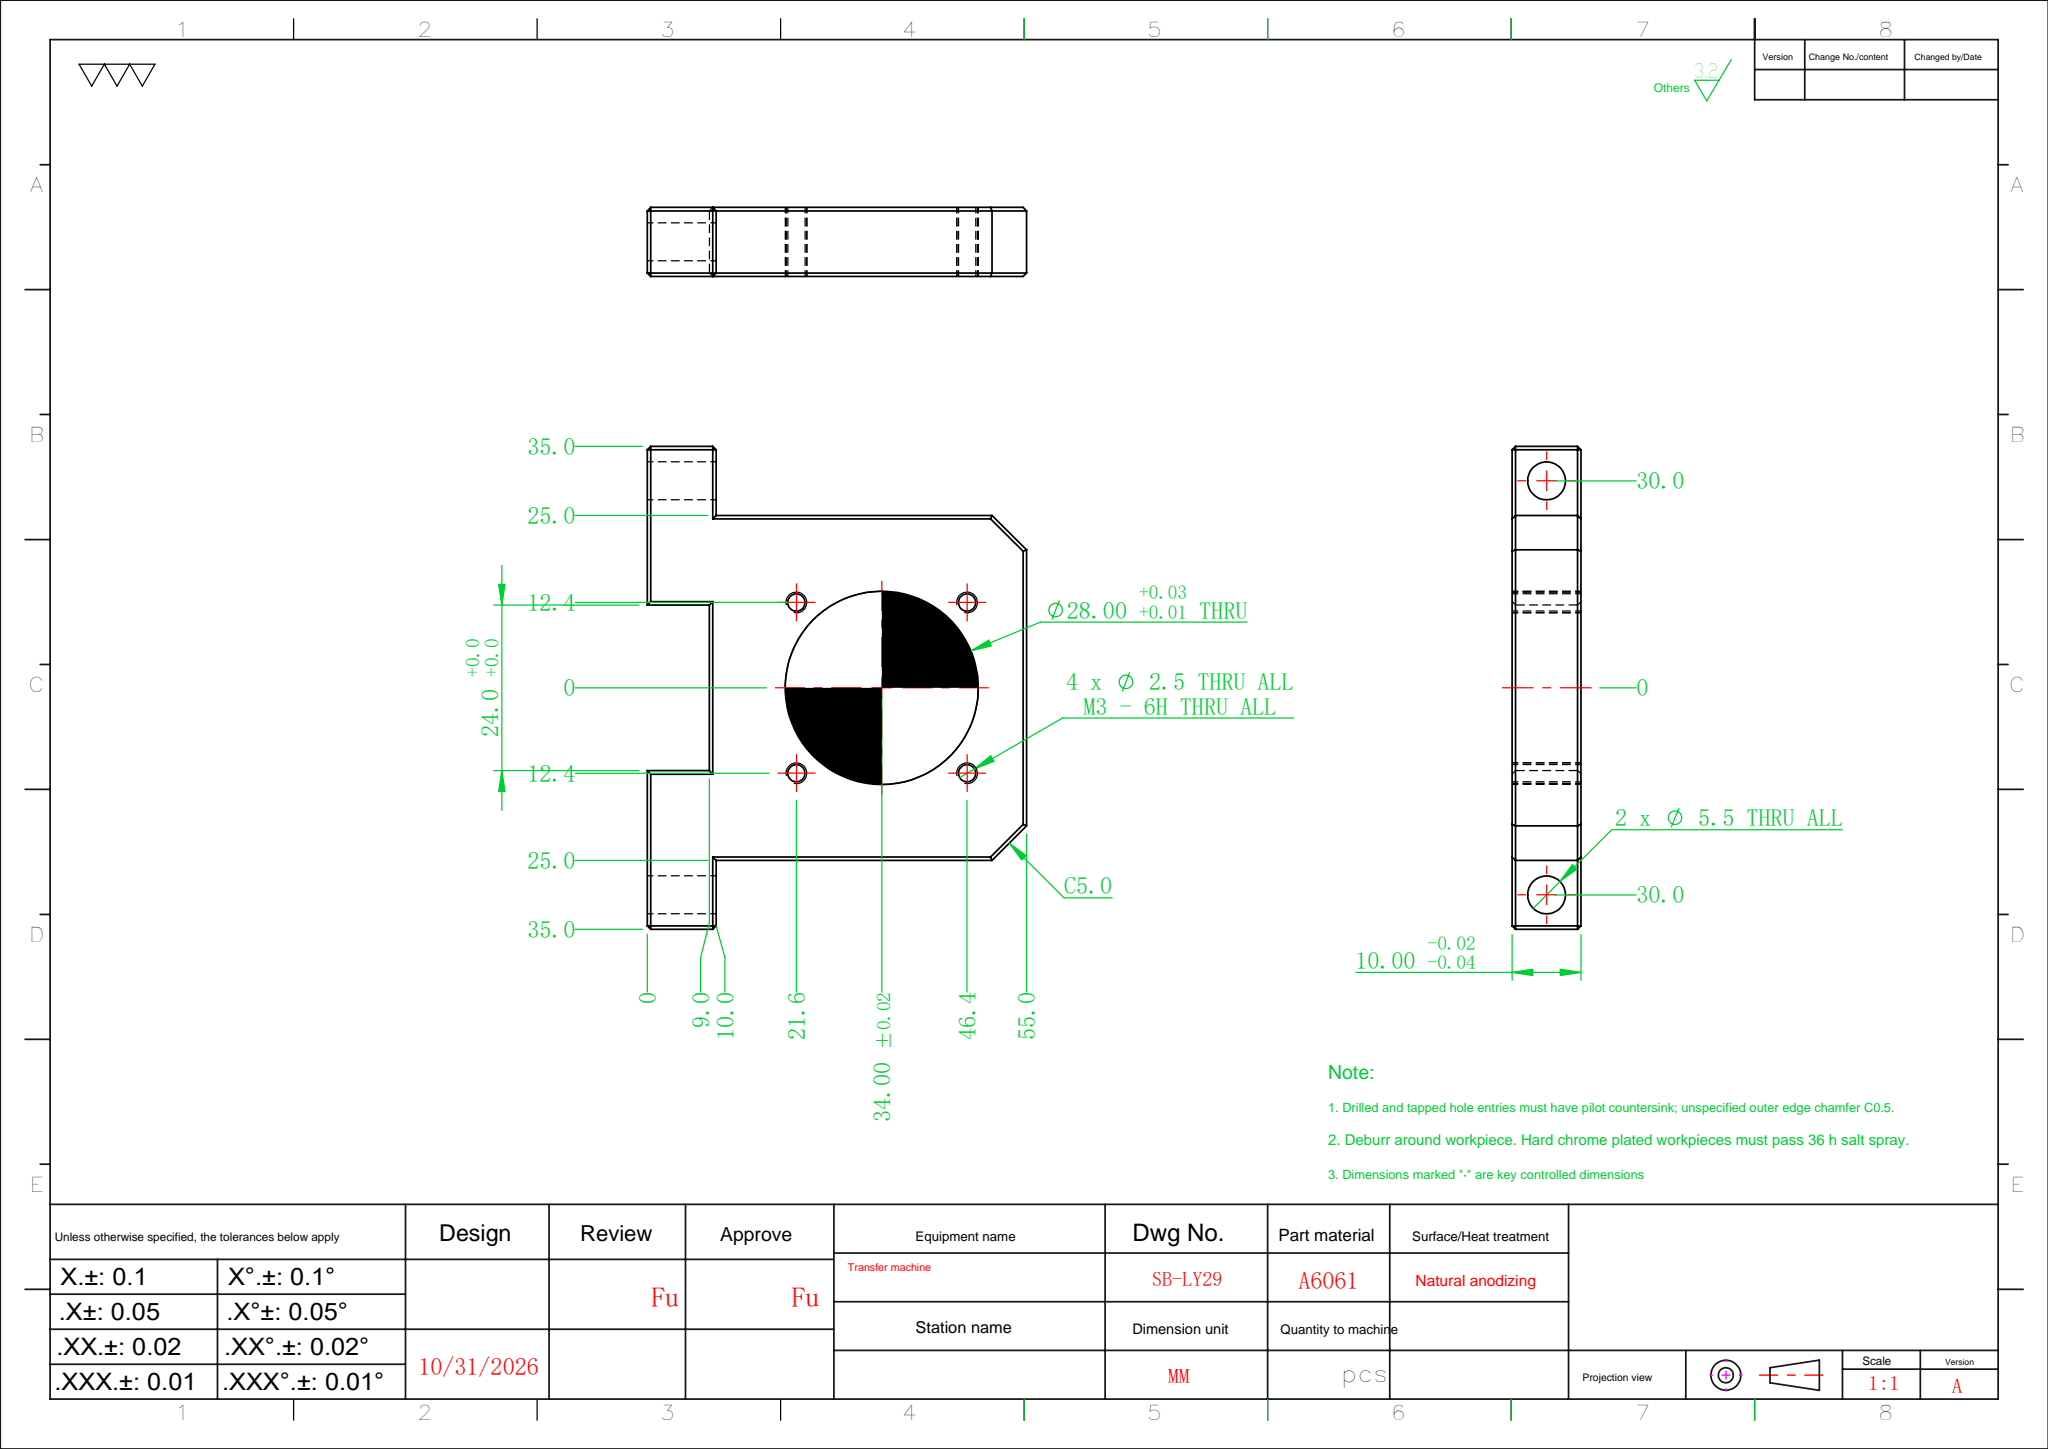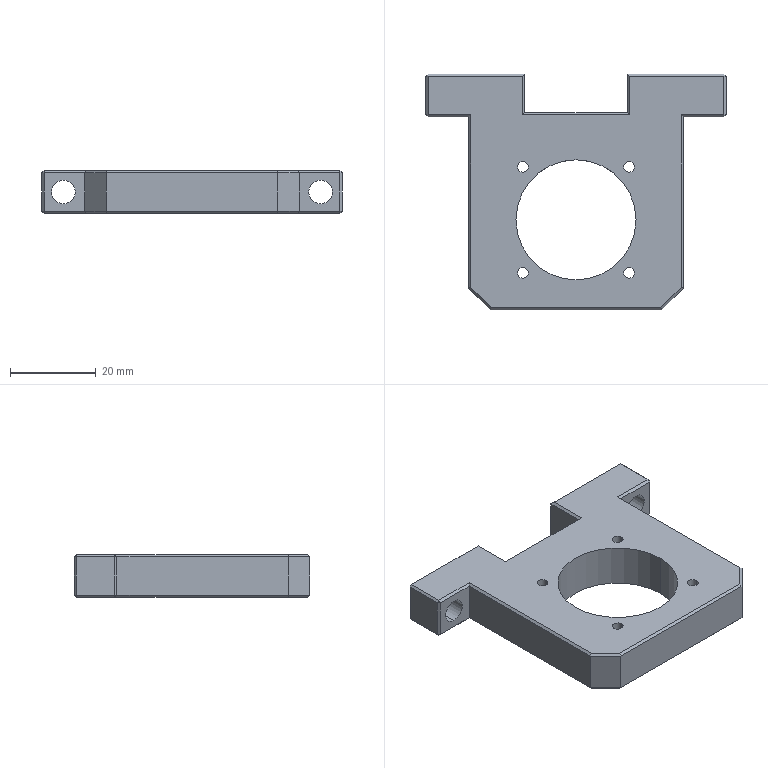Part | SolidWorks | features Chamfer 2, Cut 2, HoleWzd 2, Extrusion 1, ICE 1 | 1 solid | 70 faces | box 70 x 55 x 10 mm | volume 20191 mm3 | plane 56 | cylinder 14 | commonest cylinder face diameters 2.5 x8 5.5 x4 28 x2